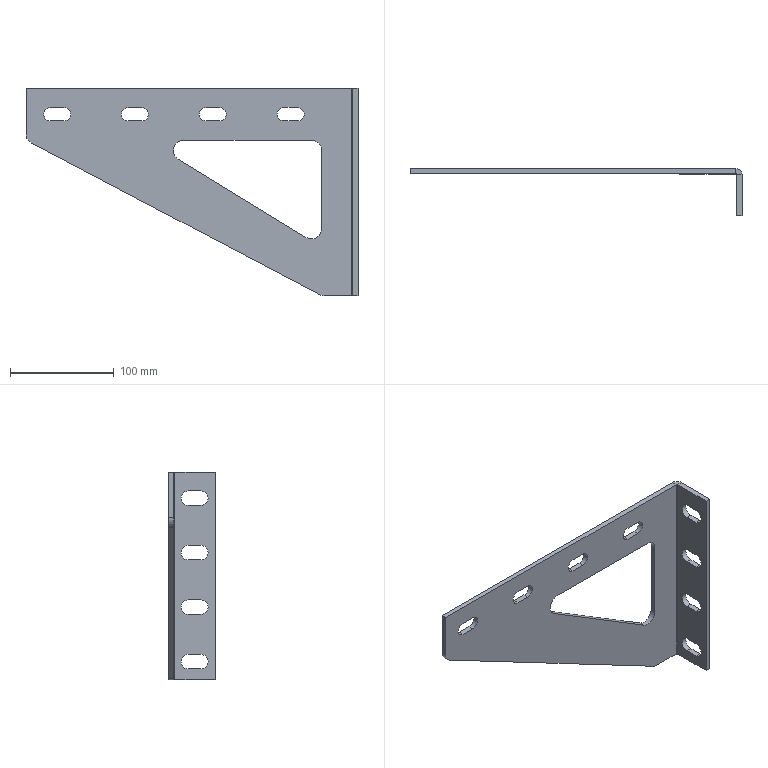Part | SolidWorks | features MirrorStock 1 | 1 solid | 59 faces | box 320 x 45 x 200 mm | volume 197310 mm3 | plane 32 | cylinder 27 | commonest cylinder face diameters 14 x12 13 x8 20 x5 2 x1 12 x1